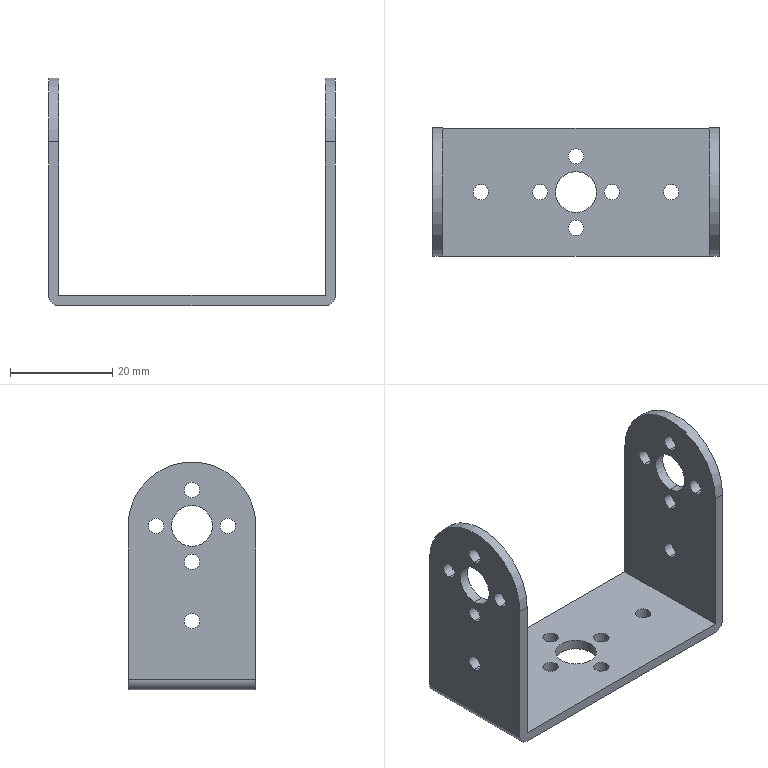Part | STEP file | U short bracket | 1 solid | 50 faces | box 56 x 25 x 44.5 mm | volume 6211 mm3 | cylinder 42 | plane 8 | commonest cylinder face diameters 3 x32 8 x6 4 x2 25 x2